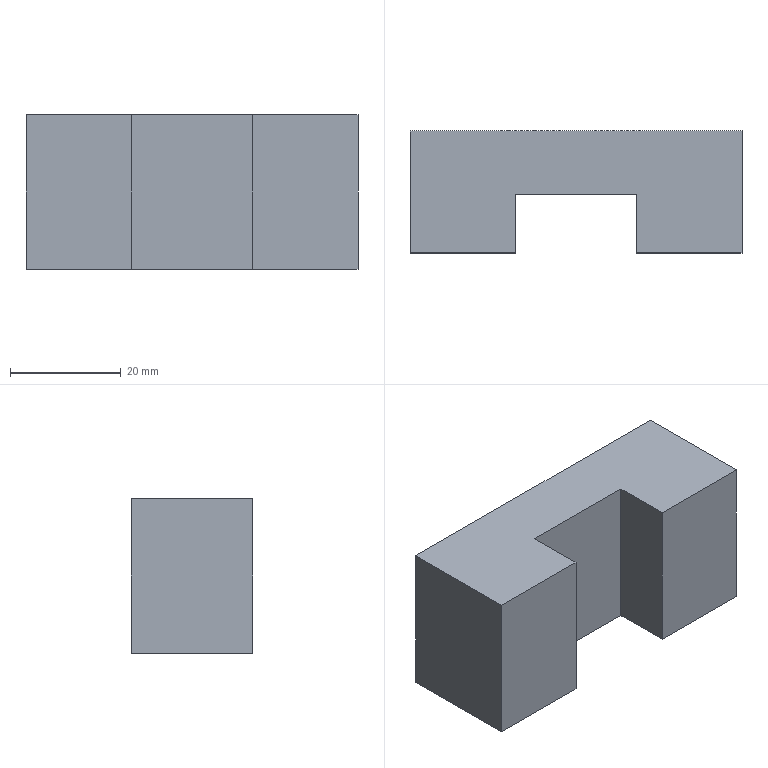Part | STEP file | Clamp-HGH20 | 1 solid | 26 faces | box 60 x 22 x 28 mm | volume 29915 mm3 | plane 10 | cylinder 8 | cone 8 | commonest cylinder face diameters 4.2 x8